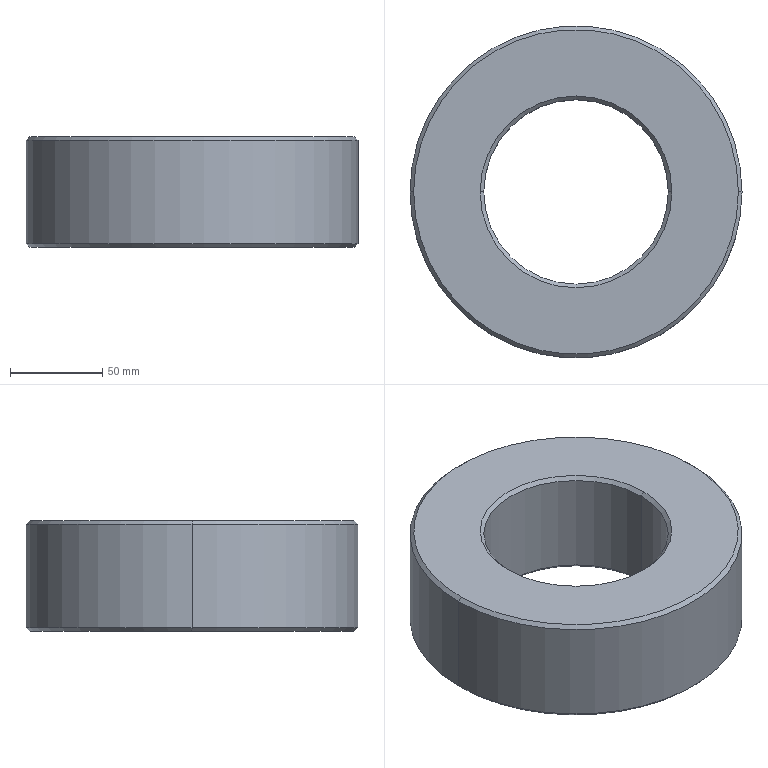Part | SolidWorks | features Chamfer 1, Extrusion 1 | 1 solid | 14 faces | box 180 x 180 x 60 mm | volume 1052057 mm3 | cone 8 | cylinder 4 | plane 2 | commonest cylinder face diameters 100 x2 180 x2
STEP:
#1=CARTESIAN_POINT('',(-50.,0.,58.));
#2=VERTEX_POINT('',#1);
#3=CARTESIAN_POINT('',(50.,0.,58.));
#4=VERTEX_POINT('',#3);
#5=CARTESIAN_POINT('',(0.,0.,58.));
#6=DIRECTION('',(0.,0.,1.));
#7=DIRECTION('',(1.,0.,0.));
#8=AXIS2_PLACEMENT_3D('',#5,#6,#7);
#9=CIRCLE('',#8,50.);
#10=EDGE_CURVE('',#2,#4,#9,.T.);
#11=ORIENTED_EDGE('',*,*,#10,.F.);
#12=CARTESIAN_POINT('',(-52.,0.,60.));
#13=VERTEX_POINT('',#12);
#14=CARTESIAN_POINT('',(-50.,0.,58.));
#15=DIRECTION('',(-0.7071,0.,0.7071));
#16=VECTOR('',#15,1000.);
#17=LINE('',#14,#16);
#18=EDGE_CURVE('',#2,#13,#17,.T.);
#19=ORIENTED_EDGE('',*,*,#18,.T.);
#20=CARTESIAN_POINT('',(52.,0.,60.));
#21=VERTEX_POINT('',#20);
#22=CARTESIAN_POINT('',(0.,0.,60.));
#23=DIRECTION('',(0.,0.,-1.));
#24=DIRECTION('',(1.,0.,0.));
#25=AXIS2_PLACEMENT_3D('',#22,#23,#24);
#26=CIRCLE('',#25,52.);
#27=EDGE_CURVE('',#21,#13,#26,.T.);
#28=ORIENTED_EDGE('',*,*,#27,.F.);
#29=CARTESIAN_POINT('',(50.,0.,58.));
#30=DIRECTION('',(0.7071,0.,0.7071));
#31=VECTOR('',#30,1000.);
#32=LINE('',#29,#31);
#33=EDGE_CURVE('',#4,#21,#32,.T.);
#34=ORIENTED_EDGE('',*,*,#33,.F.);
#35=EDGE_LOOP('',(#11,#19,#28,#34));
#36=FACE_OUTER_BOUND('',#35,.T.);
#37=CARTESIAN_POINT('',(0.,0.,58.));
#38=DIRECTION('',(0.,0.,1.));
#39=DIRECTION('',(1.,0.,0.));
#40=AXIS2_PLACEMENT_3D('',#37,#38,#39);
#41=CONICAL_SURFACE('',#40,50.,0.7854);
#42=ADVANCED_FACE('',(#36),#41,.F.);
#43=CARTESIAN_POINT('',(88.,0.,60.));
#44=VERTEX_POINT('',#43);
#45=CARTESIAN_POINT('',(-88.,0.,60.));
#46=VERTEX_POINT('',#45);
#47=CARTESIAN_POINT('',(0.,0.,60.));
#48=DIRECTION('',(0.,0.,1.));
#49=DIRECTION('',(1.,0.,0.));
#50=AXIS2_PLACEMENT_3D('',#47,#48,#49);
#51=CIRCLE('',#50,88.);
#52=EDGE_CURVE('',#44,#46,#51,.T.);
#53=ORIENTED_EDGE('',*,*,#52,.F.);
#54=CARTESIAN_POINT('',(90.,0.,58.));
#55=VERTEX_POINT('',#54);
#56=CARTESIAN_POINT('',(88.,0.,60.));
#57=DIRECTION('',(0.7071,0.,-0.7071));
#58=VECTOR('',#57,1000.);
#59=LINE('',#56,#58);
#60=EDGE_CURVE('',#44,#55,#59,.T.);
#61=ORIENTED_EDGE('',*,*,#60,.T.);
#62=CARTESIAN_POINT('',(-90.,0.,58.));
#63=VERTEX_POINT('',#62);
#64=CARTESIAN_POINT('',(0.,0.,58.));
#65=DIRECTION('',(0.,0.,-1.));
#66=DIRECTION('',(1.,0.,0.));
#67=AXIS2_PLACEMENT_3D('',#64,#65,#66);
#68=CIRCLE('',#67,90.);
#69=EDGE_CURVE('',#63,#55,#68,.T.);
#70=ORIENTED_EDGE('',*,*,#69,.F.);
#71=CARTESIAN_POINT('',(-88.,0.,60.));
#72=DIRECTION('',(-0.7071,0.,-0.7071));
#73=VECTOR('',#72,1000.);
#74=LINE('',#71,#73);
#75=EDGE_CURVE('',#46,#63,#74,.T.);
#76=ORIENTED_EDGE('',*,*,#75,.F.);
#77=EDGE_LOOP('',(#53,#61,#70,#76));
#78=FACE_OUTER_BOUND('',#77,.T.);
#79=CARTESIAN_POINT('',(0.,0.,60.));
#80=DIRECTION('',(0.,0.,-1.));
#81=DIRECTION('',(-1.,0.,0.));
#82=AXIS2_PLACEMENT_3D('',#79,#80,#81);
#83=CONICAL_SURFACE('',#82,88.,0.7854);
#84=ADVANCED_FACE('',(#78),#83,.T.);
#85=CARTESIAN_POINT('',(50.,0.,2.));
#86=VERTEX_POINT('',#85);
#87=CARTESIAN_POINT('',(-50.,0.,2.));
#88=VERTEX_POINT('',#87);
#89=CARTESIAN_POINT('',(0.,0.,2.));
#90=DIRECTION('',(0.,0.,-1.));
#91=DIRECTION('',(1.,0.,0.));
#92=AXIS2_PLACEMENT_3D('',#89,#90,#91);
#93=CIRCLE('',#92,50.);
#94=EDGE_CURVE('',#86,#88,#93,.T.);
#95=ORIENTED_EDGE('',*,*,#94,.F.);
#96=CARTESIAN_POINT('',(52.,0.,0.));
#97=VERTEX_POINT('',#96);
#98=CARTESIAN_POINT('',(52.,0.,0.));
#99=DIRECTION('',(0.7071,0.,-0.7071));
#100=VECTOR('',#99,1000.);
#101=LINE('',#98,#100);
#102=EDGE_CURVE('',#86,#97,#101,.T.);
#103=ORIENTED_EDGE('',*,*,#102,.T.);
#104=CARTESIAN_POINT('',(-52.,0.,0.));
#105=VERTEX_POINT('',#104);
#106=CARTESIAN_POINT('',(0.,0.,0.));
#107=DIRECTION('',(0.,0.,1.));
#108=DIRECTION('',(1.,0.,0.));
#109=AXIS2_PLACEMENT_3D('',#106,#107,#108);
#110=CIRCLE('',#109,52.);
#111=EDGE_CURVE('',#105,#97,#110,.T.);
#112=ORIENTED_EDGE('',*,*,#111,.F.);
#113=CARTESIAN_POINT('',(-52.,0.,0.));
#114=DIRECTION('',(-0.7071,0.,-0.7071));
#115=VECTOR('',#114,1000.);
#116=LINE('',#113,#115);
#117=EDGE_CURVE('',#88,#105,#116,.T.);
#118=ORIENTED_EDGE('',*,*,#117,.F.);
#119=EDGE_LOOP('',(#95,#103,#112,#118));
#120=FACE_OUTER_BOUND('',#119,.T.);
#121=CARTESIAN_POINT('',(0.,0.,0.));
#122=DIRECTION('',(0.,0.,-1.));
#123=DIRECTION('',(-1.,0.,0.));
#124=AXIS2_PLACEMENT_3D('',#121,#122,#123);
#125=CONICAL_SURFACE('',#124,52.,0.7854);
#126=ADVANCED_FACE('',(#120),#125,.F.);
#127=CARTESIAN_POINT('',(-88.,0.,0.));
#128=VERTEX_POINT('',#127);
#129=CARTESIAN_POINT('',(88.,0.,0.));
#130=VERTEX_POINT('',#129);
#131=CARTESIAN_POINT('',(0.,0.,0.));
#132=DIRECTION('',(0.,0.,-1.));
#133=DIRECTION('',(1.,0.,0.));
#134=AXIS2_PLACEMENT_3D('',#131,#132,#133);
#135=CIRCLE('',#134,88.);
#136=EDGE_CURVE('',#128,#130,#135,.T.);
#137=ORIENTED_EDGE('',*,*,#136,.F.);
#138=CARTESIAN_POINT('',(-90.,0.,2.));
#139=VERTEX_POINT('',#138);
#140=CARTESIAN_POINT('',(-90.,0.,2.));
#141=DIRECTION('',(-0.7071,0.,0.7071));
#142=VECTOR('',#141,1000.);
#143=LINE('',#140,#142);
#144=EDGE_CURVE('',#128,#139,#143,.T.);
#145=ORIENTED_EDGE('',*,*,#144,.T.);
#146=CARTESIAN_POINT('',(90.,0.,2.));
#147=VERTEX_POINT('',#146);
#148=CARTESIAN_POINT('',(0.,0.,2.));
#149=DIRECTION('',(0.,0.,1.));
#150=DIRECTION('',(1.,0.,0.));
#151=AXIS2_PLACEMENT_3D('',#148,#149,#150);
#152=CIRCLE('',#151,90.);
#153=EDGE_CURVE('',#147,#139,#152,.T.);
#154=ORIENTED_EDGE('',*,*,#153,.F.);
#155=CARTESIAN_POINT('',(90.,0.,2.));
#156=DIRECTION('',(0.7071,0.,0.7071));
#157=VECTOR('',#156,1000.);
#158=LINE('',#155,#157);
#159=EDGE_CURVE('',#130,#147,#158,.T.);
#160=ORIENTED_EDGE('',*,*,#159,.F.);
#161=EDGE_LOOP('',(#137,#145,#154,#160));
#162=FACE_OUTER_BOUND('',#161,.T.);
#163=CARTESIAN_POINT('',(0.,0.,2.));
#164=DIRECTION('',(0.,0.,1.));
#165=DIRECTION('',(1.,0.,0.));
#166=AXIS2_PLACEMENT_3D('',#163,#164,#165);
#167=CONICAL_SURFACE('',#166,90.,0.7854);
#168=ADVANCED_FACE('',(#162),#167,.T.);
#169=ORIENTED_EDGE('',*,*,#10,.T.);
#170=CARTESIAN_POINT('',(50.,0.,60.));
#171=DIRECTION('',(0.,0.,-1.));
#172=VECTOR('',#171,1000.);
#173=LINE('',#170,#172);
#174=EDGE_CURVE('',#4,#86,#173,.T.);
#175=ORIENTED_EDGE('',*,*,#174,.T.);
#176=ORIENTED_EDGE('',*,*,#94,.T.);
#177=CARTESIAN_POINT('',(-50.,0.,60.));
#178=DIRECTION('',(0.,0.,-1.));
#179=VECTOR('',#178,1000.);
#180=LINE('',#177,#179);
#181=EDGE_CURVE('',#2,#88,#180,.T.);
#182=ORIENTED_EDGE('',*,*,#181,.F.);
#183=EDGE_LOOP('',(#169,#175,#176,#182));
#184=FACE_OUTER_BOUND('',#183,.T.);
#185=CARTESIAN_POINT('',(0.,0.,60.));
#186=DIRECTION('',(0.,0.,-1.));
#187=DIRECTION('',(-1.,0.,0.));
#188=AXIS2_PLACEMENT_3D('',#185,#186,#187);
#189=CYLINDRICAL_SURFACE('',#188,50.);
#190=ADVANCED_FACE('',(#184),#189,.F.);
#191=ORIENTED_EDGE('',*,*,#69,.T.);
#192=CARTESIAN_POINT('',(90.,0.,60.));
#193=DIRECTION('',(0.,0.,-1.));
#194=VECTOR('',#193,1000.);
#195=LINE('',#192,#194);
#196=EDGE_CURVE('',#55,#147,#195,.T.);
#197=ORIENTED_EDGE('',*,*,#196,.T.);
#198=ORIENTED_EDGE('',*,*,#153,.T.);
#199=CARTESIAN_POINT('',(-90.,0.,60.));
#200=DIRECTION('',(0.,0.,-1.));
#201=VECTOR('',#200,1000.);
#202=LINE('',#199,#201);
#203=EDGE_CURVE('',#63,#139,#202,.T.);
#204=ORIENTED_EDGE('',*,*,#203,.F.);
#205=EDGE_LOOP('',(#191,#197,#198,#204));
#206=FACE_OUTER_BOUND('',#205,.T.);
#207=CARTESIAN_POINT('',(0.,0.,60.));
#208=DIRECTION('',(0.,0.,-1.));
#209=DIRECTION('',(-1.,0.,0.));
#210=AXIS2_PLACEMENT_3D('',#207,#208,#209);
#211=CYLINDRICAL_SURFACE('',#210,90.);
#212=ADVANCED_FACE('',(#206),#211,.T.);
#213=CARTESIAN_POINT('',(0.,0.,60.));
#214=DIRECTION('',(0.,0.,1.));
#215=DIRECTION('',(1.,0.,0.));
#216=AXIS2_PLACEMENT_3D('',#213,#214,#215);
#217=CIRCLE('',#216,88.);
#218=EDGE_CURVE('',#46,#44,#217,.T.);
#219=ORIENTED_EDGE('',*,*,#218,.T.);
#220=ORIENTED_EDGE('',*,*,#52,.T.);
#221=EDGE_LOOP('',(#219,#220));
#222=FACE_OUTER_BOUND('',#221,.T.);
#223=ORIENTED_EDGE('',*,*,#27,.T.);
#224=CARTESIAN_POINT('',(0.,0.,60.));
#225=DIRECTION('',(0.,0.,-1.));
#226=DIRECTION('',(1.,0.,0.));
#227=AXIS2_PLACEMENT_3D('',#224,#225,#226);
#228=CIRCLE('',#227,52.);
#229=EDGE_CURVE('',#13,#21,#228,.T.);
#230=ORIENTED_EDGE('',*,*,#229,.T.);
#231=EDGE_LOOP('',(#223,#230));
#232=FACE_BOUND('',#231,.T.);
#233=CARTESIAN_POINT('',(0.,0.,60.));
#234=DIRECTION('',(0.,0.,1.));
#235=DIRECTION('',(1.,0.,0.));
#236=AXIS2_PLACEMENT_3D('',#233,#234,#235);
#237=PLANE('',#236);
#238=ADVANCED_FACE('',(#222,#232),#237,.T.);
#239=CARTESIAN_POINT('',(0.,0.,0.));
#240=DIRECTION('',(0.,0.,-1.));
#241=DIRECTION('',(1.,0.,0.));
#242=AXIS2_PLACEMENT_3D('',#239,#240,#241);
#243=CIRCLE('',#242,88.);
#244=EDGE_CURVE('',#130,#128,#243,.T.);
#245=ORIENTED_EDGE('',*,*,#244,.T.);
#246=ORIENTED_EDGE('',*,*,#136,.T.);
#247=EDGE_LOOP('',(#245,#246));
#248=FACE_OUTER_BOUND('',#247,.T.);
#249=ORIENTED_EDGE('',*,*,#111,.T.);
#250=CARTESIAN_POINT('',(0.,0.,0.));
#251=DIRECTION('',(0.,0.,1.));
#252=DIRECTION('',(1.,0.,0.));
#253=AXIS2_PLACEMENT_3D('',#250,#251,#252);
#254=CIRCLE('',#253,52.);
#255=EDGE_CURVE('',#97,#105,#254,.T.);
#256=ORIENTED_EDGE('',*,*,#255,.T.);
#257=EDGE_LOOP('',(#249,#256));
#258=FACE_BOUND('',#257,.T.);
#259=CARTESIAN_POINT('',(0.,0.,0.));
#260=DIRECTION('',(0.,0.,1.));
#261=DIRECTION('',(1.,0.,0.));
#262=AXIS2_PLACEMENT_3D('',#259,#260,#261);
#263=PLANE('',#262);
#264=ADVANCED_FACE('',(#248,#258),#263,.F.);
#265=ORIENTED_EDGE('',*,*,#196,.F.);
#266=CARTESIAN_POINT('',(0.,0.,58.));
#267=DIRECTION('',(0.,0.,-1.));
#268=DIRECTION('',(1.,0.,0.));
#269=AXIS2_PLACEMENT_3D('',#266,#267,#268);
#270=CIRCLE('',#269,90.);
#271=EDGE_CURVE('',#55,#63,#270,.T.);
#272=ORIENTED_EDGE('',*,*,#271,.T.);
#273=ORIENTED_EDGE('',*,*,#203,.T.);
#274=CARTESIAN_POINT('',(0.,0.,2.));
#275=DIRECTION('',(0.,0.,1.));
#276=DIRECTION('',(1.,0.,0.));
#277=AXIS2_PLACEMENT_3D('',#274,#275,#276);
#278=CIRCLE('',#277,90.);
#279=EDGE_CURVE('',#139,#147,#278,.T.);
#280=ORIENTED_EDGE('',*,*,#279,.T.);
#281=EDGE_LOOP('',(#265,#272,#273,#280));
#282=FACE_OUTER_BOUND('',#281,.T.);
#283=CARTESIAN_POINT('',(0.,0.,60.));
#284=DIRECTION('',(0.,0.,-1.));
#285=DIRECTION('',(-1.,0.,0.));
#286=AXIS2_PLACEMENT_3D('',#283,#284,#285);
#287=CYLINDRICAL_SURFACE('',#286,90.);
#288=ADVANCED_FACE('',(#282),#287,.T.);
#289=ORIENTED_EDGE('',*,*,#174,.F.);
#290=CARTESIAN_POINT('',(0.,0.,58.));
#291=DIRECTION('',(0.,0.,1.));
#292=DIRECTION('',(1.,0.,0.));
#293=AXIS2_PLACEMENT_3D('',#290,#291,#292);
#294=CIRCLE('',#293,50.);
#295=EDGE_CURVE('',#4,#2,#294,.T.);
#296=ORIENTED_EDGE('',*,*,#295,.T.);
#297=ORIENTED_EDGE('',*,*,#181,.T.);
#298=CARTESIAN_POINT('',(0.,0.,2.));
#299=DIRECTION('',(0.,0.,-1.));
#300=DIRECTION('',(1.,0.,0.));
#301=AXIS2_PLACEMENT_3D('',#298,#299,#300);
#302=CIRCLE('',#301,50.);
#303=EDGE_CURVE('',#88,#86,#302,.T.);
#304=ORIENTED_EDGE('',*,*,#303,.T.);
#305=EDGE_LOOP('',(#289,#296,#297,#304));
#306=FACE_OUTER_BOUND('',#305,.T.);
#307=CARTESIAN_POINT('',(0.,0.,60.));
#308=DIRECTION('',(0.,0.,-1.));
#309=DIRECTION('',(-1.,0.,0.));
#310=AXIS2_PLACEMENT_3D('',#307,#308,#309);
#311=CYLINDRICAL_SURFACE('',#310,50.);
#312=ADVANCED_FACE('',(#306),#311,.F.);
#313=ORIENTED_EDGE('',*,*,#144,.F.);
#314=ORIENTED_EDGE('',*,*,#244,.F.);
#315=ORIENTED_EDGE('',*,*,#159,.T.);
#316=ORIENTED_EDGE('',*,*,#279,.F.);
#317=EDGE_LOOP('',(#313,#314,#315,#316));
#318=FACE_OUTER_BOUND('',#317,.T.);
#319=CARTESIAN_POINT('',(0.,0.,2.));
#320=DIRECTION('',(0.,0.,1.));
#321=DIRECTION('',(1.,0.,0.));
#322=AXIS2_PLACEMENT_3D('',#319,#320,#321);
#323=CONICAL_SURFACE('',#322,90.,0.7854);
#324=ADVANCED_FACE('',(#318),#323,.T.);
#325=ORIENTED_EDGE('',*,*,#102,.F.);
#326=ORIENTED_EDGE('',*,*,#303,.F.);
#327=ORIENTED_EDGE('',*,*,#117,.T.);
#328=ORIENTED_EDGE('',*,*,#255,.F.);
#329=EDGE_LOOP('',(#325,#326,#327,#328));
#330=FACE_OUTER_BOUND('',#329,.T.);
#331=CARTESIAN_POINT('',(0.,0.,0.));
#332=DIRECTION('',(0.,0.,-1.));
#333=DIRECTION('',(-1.,0.,0.));
#334=AXIS2_PLACEMENT_3D('',#331,#332,#333);
#335=CONICAL_SURFACE('',#334,52.,0.7854);
#336=ADVANCED_FACE('',(#330),#335,.F.);
#337=ORIENTED_EDGE('',*,*,#60,.F.);
#338=ORIENTED_EDGE('',*,*,#218,.F.);
#339=ORIENTED_EDGE('',*,*,#75,.T.);
#340=ORIENTED_EDGE('',*,*,#271,.F.);
#341=EDGE_LOOP('',(#337,#338,#339,#340));
#342=FACE_OUTER_BOUND('',#341,.T.);
#343=CARTESIAN_POINT('',(0.,0.,60.));
#344=DIRECTION('',(0.,0.,-1.));
#345=DIRECTION('',(-1.,0.,0.));
#346=AXIS2_PLACEMENT_3D('',#343,#344,#345);
#347=CONICAL_SURFACE('',#346,88.,0.7854);
#348=ADVANCED_FACE('',(#342),#347,.T.);
#349=ORIENTED_EDGE('',*,*,#18,.F.);
#350=ORIENTED_EDGE('',*,*,#295,.F.);
#351=ORIENTED_EDGE('',*,*,#33,.T.);
#352=ORIENTED_EDGE('',*,*,#229,.F.);
#353=EDGE_LOOP('',(#349,#350,#351,#352));
#354=FACE_OUTER_BOUND('',#353,.T.);
#355=CARTESIAN_POINT('',(0.,0.,58.));
#356=DIRECTION('',(0.,0.,1.));
#357=DIRECTION('',(1.,0.,0.));
#358=AXIS2_PLACEMENT_3D('',#355,#356,#357);
#359=CONICAL_SURFACE('',#358,50.,0.7854);
#360=ADVANCED_FACE('',(#354),#359,.F.);
#361=CLOSED_SHELL('',(#42,#84,#126,#168,#190,#212,#238,#264,#288,#312,#324,#336,#348,#360));
#362=MANIFOLD_SOLID_BREP('',#361);
#363=CARTESIAN_POINT('',(0.,0.,0.));
#364=DIRECTION('',(0.,0.,1.));
#365=DIRECTION('',(1.,0.,0.));
#366=AXIS2_PLACEMENT_3D('',#363,#364,#365);
#367=(LENGTH_UNIT()NAMED_UNIT(*)SI_UNIT(.MILLI.,.METRE.));
#368=UNCERTAINTY_MEASURE_WITH_UNIT(LENGTH_MEASURE(0.00001),#367,'','');
#369=(NAMED_UNIT(*)PLANE_ANGLE_UNIT()SI_UNIT($,.RADIAN.));
#370=(NAMED_UNIT(*)SI_UNIT($,.STERADIAN.)SOLID_ANGLE_UNIT());
#371=(GEOMETRIC_REPRESENTATION_CONTEXT(3)GLOBAL_UNCERTAINTY_ASSIGNED_CONTEXT((#368))GLOBAL_UNIT_ASSIGNED_CONTEXT((#367,#369,#370))REPRESENTATION_CONTEXT('',''));
#372=ADVANCED_BREP_SHAPE_REPRESENTATION('',(#362,#366),#371);